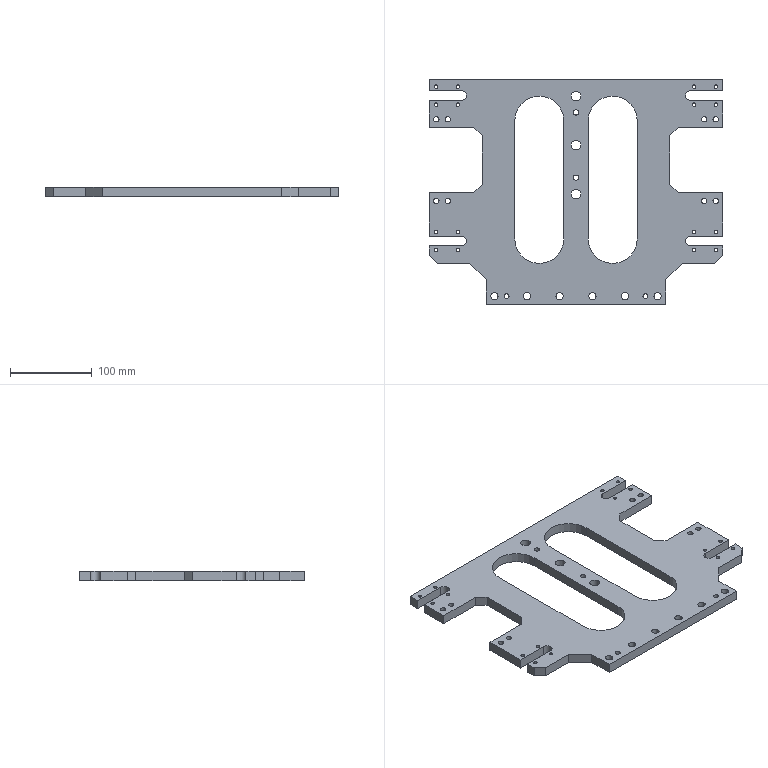Part | 1 solid | 87 faces | box 360 x 275 x 12 mm | volume 666691 mm3 | cylinder 45 | plane 42 | commonest cylinder face diameters 4.2 x16 6.6 x10 12 x7 9 x6 60 x4 6 x2